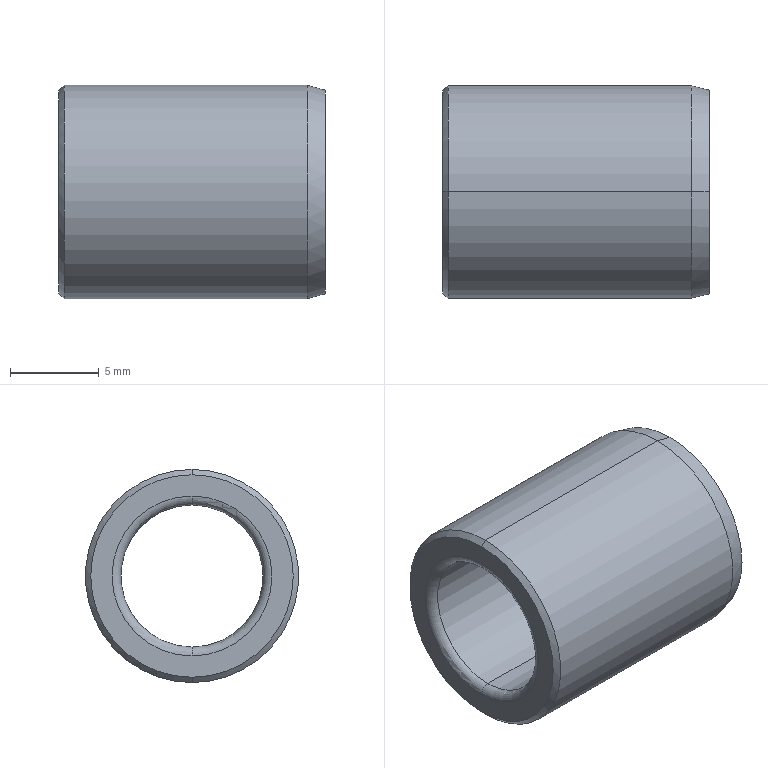Part | NX | features BREP 1 | 1 solid | 14 faces | box 15 x 12 x 12 mm | volume 933.062 mm3 | cylinder 4 | cone 4 | torus 4 | plane 2 | commonest cylinder face diameters 8 x2 12 x2
STEP:
#1=CARTESIAN_POINT('',(14.,0.,6.));
#2=VERTEX_POINT('',#1);
#3=CARTESIAN_POINT('',(14.,0.,-6.));
#4=VERTEX_POINT('',#3);
#5=CARTESIAN_POINT('',(14.,0.,0.));
#6=DIRECTION('',(-1.,0.,0.));
#7=DIRECTION('',(0.,0.,1.));
#8=AXIS2_PLACEMENT_3D('',#5,#6,#7);
#9=CIRCLE('',#8,6.);
#10=EDGE_CURVE('',#2,#4,#9,.T.);
#11=ORIENTED_EDGE('',*,*,#10,.T.);
#12=CARTESIAN_POINT('',(0.3,0.,-6.));
#13=VERTEX_POINT('',#12);
#14=CARTESIAN_POINT('',(15.,0.,-6.));
#15=DIRECTION('',(-1.,0.,0.));
#16=VECTOR('',#15,1000.);
#17=LINE('',#14,#16);
#18=EDGE_CURVE('',#13,#4,#17,.F.);
#19=ORIENTED_EDGE('',*,*,#18,.F.);
#20=CARTESIAN_POINT('',(0.3,0.,6.));
#21=VERTEX_POINT('',#20);
#22=CARTESIAN_POINT('',(0.3,0.,0.));
#23=DIRECTION('',(-1.,0.,0.));
#24=DIRECTION('',(0.,0.,1.));
#25=AXIS2_PLACEMENT_3D('',#22,#23,#24);
#26=CIRCLE('',#25,6.);
#27=EDGE_CURVE('',#21,#13,#26,.T.);
#28=ORIENTED_EDGE('',*,*,#27,.F.);
#29=CARTESIAN_POINT('',(15.,0.,6.));
#30=DIRECTION('',(-1.,0.,0.));
#31=VECTOR('',#30,1000.);
#32=LINE('',#29,#31);
#33=EDGE_CURVE('',#21,#2,#32,.F.);
#34=ORIENTED_EDGE('',*,*,#33,.T.);
#35=EDGE_LOOP('',(#11,#19,#28,#34));
#36=FACE_BOUND('',#35,.T.);
#37=CARTESIAN_POINT('',(15.,0.,0.));
#38=DIRECTION('',(-1.,0.,0.));
#39=DIRECTION('',(0.,0.,1.));
#40=AXIS2_PLACEMENT_3D('',#37,#38,#39);
#41=CYLINDRICAL_SURFACE('',#40,6.);
#42=ADVANCED_FACE('',(#36),#41,.T.);
#43=CARTESIAN_POINT('',(15.,0.,5.732));
#44=VERTEX_POINT('',#43);
#45=CARTESIAN_POINT('',(15.,0.,-5.732));
#46=VERTEX_POINT('',#45);
#47=CARTESIAN_POINT('',(15.,0.,0.));
#48=DIRECTION('',(-1.,0.,0.));
#49=DIRECTION('',(0.,0.,1.));
#50=AXIS2_PLACEMENT_3D('',#47,#48,#49);
#51=CIRCLE('',#50,5.732);
#52=EDGE_CURVE('',#44,#46,#51,.T.);
#53=ORIENTED_EDGE('',*,*,#52,.T.);
#54=CARTESIAN_POINT('',(15.,0.,-5.732));
#55=DIRECTION('',(-0.9659,0.,-0.2588));
#56=VECTOR('',#55,1000.);
#57=LINE('',#54,#56);
#58=EDGE_CURVE('',#4,#46,#57,.F.);
#59=ORIENTED_EDGE('',*,*,#58,.F.);
#60=ORIENTED_EDGE('',*,*,#10,.F.);
#61=CARTESIAN_POINT('',(15.,0.,5.732));
#62=DIRECTION('',(-0.9659,0.,0.2588));
#63=VECTOR('',#62,1000.);
#64=LINE('',#61,#63);
#65=EDGE_CURVE('',#2,#44,#64,.F.);
#66=ORIENTED_EDGE('',*,*,#65,.T.);
#67=EDGE_LOOP('',(#53,#59,#60,#66));
#68=FACE_BOUND('',#67,.T.);
#69=CARTESIAN_POINT('',(15.,0.,0.));
#70=DIRECTION('',(-1.,0.,0.));
#71=DIRECTION('',(0.,0.,1.));
#72=AXIS2_PLACEMENT_3D('',#69,#70,#71);
#73=CONICAL_SURFACE('',#72,5.732,0.2618);
#74=ADVANCED_FACE('',(#68),#73,.T.);
#75=CARTESIAN_POINT('',(14.5,0.,4.));
#76=VERTEX_POINT('',#75);
#77=CARTESIAN_POINT('',(14.5,0.,-4.));
#78=VERTEX_POINT('',#77);
#79=CARTESIAN_POINT('',(14.5,0.,0.));
#80=DIRECTION('',(-1.,0.,0.));
#81=DIRECTION('',(0.,0.,1.));
#82=AXIS2_PLACEMENT_3D('',#79,#80,#81);
#83=CIRCLE('',#82,4.);
#84=EDGE_CURVE('',#76,#78,#83,.T.);
#85=ORIENTED_EDGE('',*,*,#84,.T.);
#86=CARTESIAN_POINT('',(15.,0.,-4.5));
#87=VERTEX_POINT('',#86);
#88=CARTESIAN_POINT('',(14.5,0.,-4.5));
#89=DIRECTION('',(0.,1.,0.));
#90=DIRECTION('',(0.,0.,1.));
#91=AXIS2_PLACEMENT_3D('',#88,#89,#90);
#92=CIRCLE('',#91,0.5);
#93=EDGE_CURVE('',#87,#78,#92,.F.);
#94=ORIENTED_EDGE('',*,*,#93,.F.);
#95=CARTESIAN_POINT('',(15.,0.,4.5));
#96=VERTEX_POINT('',#95);
#97=CARTESIAN_POINT('',(15.,0.,0.));
#98=DIRECTION('',(-1.,0.,0.));
#99=DIRECTION('',(0.,0.,1.));
#100=AXIS2_PLACEMENT_3D('',#97,#98,#99);
#101=CIRCLE('',#100,4.5);
#102=EDGE_CURVE('',#96,#87,#101,.T.);
#103=ORIENTED_EDGE('',*,*,#102,.F.);
#104=CARTESIAN_POINT('',(14.5,0.,4.5));
#105=DIRECTION('',(0.,-1.,0.));
#106=DIRECTION('',(0.,0.,-1.));
#107=AXIS2_PLACEMENT_3D('',#104,#105,#106);
#108=CIRCLE('',#107,0.5);
#109=EDGE_CURVE('',#96,#76,#108,.F.);
#110=ORIENTED_EDGE('',*,*,#109,.T.);
#111=EDGE_LOOP('',(#85,#94,#103,#110));
#112=FACE_BOUND('',#111,.T.);
#113=CARTESIAN_POINT('',(14.5,0.,0.));
#114=DIRECTION('',(-1.,0.,0.));
#115=DIRECTION('',(0.,0.,1.));
#116=AXIS2_PLACEMENT_3D('',#113,#114,#115);
#117=TOROIDAL_SURFACE('',#116,4.5,0.5);
#118=ADVANCED_FACE('',(#112),#117,.T.);
#119=CARTESIAN_POINT('',(14.5,0.,0.));
#120=DIRECTION('',(-1.,0.,0.));
#121=DIRECTION('',(0.,0.,1.));
#122=AXIS2_PLACEMENT_3D('',#119,#120,#121);
#123=CIRCLE('',#122,4.);
#124=EDGE_CURVE('',#78,#76,#123,.T.);
#125=ORIENTED_EDGE('',*,*,#124,.F.);
#126=CARTESIAN_POINT('',(0.5,0.,-4.));
#127=VERTEX_POINT('',#126);
#128=CARTESIAN_POINT('',(15.,0.,-4.));
#129=DIRECTION('',(-1.,0.,0.));
#130=VECTOR('',#129,1000.);
#131=LINE('',#128,#130);
#132=EDGE_CURVE('',#127,#78,#131,.F.);
#133=ORIENTED_EDGE('',*,*,#132,.F.);
#134=CARTESIAN_POINT('',(0.5,0.,4.));
#135=VERTEX_POINT('',#134);
#136=CARTESIAN_POINT('',(0.5,0.,0.));
#137=DIRECTION('',(-1.,0.,0.));
#138=DIRECTION('',(0.,0.,1.));
#139=AXIS2_PLACEMENT_3D('',#136,#137,#138);
#140=CIRCLE('',#139,4.);
#141=EDGE_CURVE('',#127,#135,#140,.T.);
#142=ORIENTED_EDGE('',*,*,#141,.T.);
#143=CARTESIAN_POINT('',(15.,0.,4.));
#144=DIRECTION('',(-1.,0.,0.));
#145=VECTOR('',#144,1000.);
#146=LINE('',#143,#145);
#147=EDGE_CURVE('',#135,#76,#146,.F.);
#148=ORIENTED_EDGE('',*,*,#147,.T.);
#149=EDGE_LOOP('',(#125,#133,#142,#148));
#150=FACE_BOUND('',#149,.T.);
#151=CARTESIAN_POINT('',(15.,0.,0.));
#152=DIRECTION('',(-1.,0.,0.));
#153=DIRECTION('',(0.,0.,1.));
#154=AXIS2_PLACEMENT_3D('',#151,#152,#153);
#155=CYLINDRICAL_SURFACE('',#154,4.);
#156=ADVANCED_FACE('',(#150),#155,.F.);
#157=CARTESIAN_POINT('',(0.,0.,4.5));
#158=VERTEX_POINT('',#157);
#159=CARTESIAN_POINT('',(0.,0.,-4.5));
#160=VERTEX_POINT('',#159);
#161=CARTESIAN_POINT('',(0.,0.,0.));
#162=DIRECTION('',(-1.,0.,0.));
#163=DIRECTION('',(0.,0.,1.));
#164=AXIS2_PLACEMENT_3D('',#161,#162,#163);
#165=CIRCLE('',#164,4.5);
#166=EDGE_CURVE('',#158,#160,#165,.T.);
#167=ORIENTED_EDGE('',*,*,#166,.T.);
#168=CARTESIAN_POINT('',(0.5,0.,-4.5));
#169=DIRECTION('',(0.,1.,0.));
#170=DIRECTION('',(0.,0.,1.));
#171=AXIS2_PLACEMENT_3D('',#168,#169,#170);
#172=CIRCLE('',#171,0.5);
#173=EDGE_CURVE('',#127,#160,#172,.F.);
#174=ORIENTED_EDGE('',*,*,#173,.F.);
#175=CARTESIAN_POINT('',(0.5,0.,0.));
#176=DIRECTION('',(-1.,0.,0.));
#177=DIRECTION('',(0.,0.,1.));
#178=AXIS2_PLACEMENT_3D('',#175,#176,#177);
#179=CIRCLE('',#178,4.);
#180=EDGE_CURVE('',#135,#127,#179,.T.);
#181=ORIENTED_EDGE('',*,*,#180,.F.);
#182=CARTESIAN_POINT('',(0.5,0.,4.5));
#183=DIRECTION('',(0.,-1.,0.));
#184=DIRECTION('',(0.,0.,-1.));
#185=AXIS2_PLACEMENT_3D('',#182,#183,#184);
#186=CIRCLE('',#185,0.5);
#187=EDGE_CURVE('',#135,#158,#186,.F.);
#188=ORIENTED_EDGE('',*,*,#187,.T.);
#189=EDGE_LOOP('',(#167,#174,#181,#188));
#190=FACE_BOUND('',#189,.T.);
#191=CARTESIAN_POINT('',(0.5,0.,0.));
#192=DIRECTION('',(-1.,0.,0.));
#193=DIRECTION('',(0.,0.,1.));
#194=AXIS2_PLACEMENT_3D('',#191,#192,#193);
#195=TOROIDAL_SURFACE('',#194,4.5,0.5);
#196=ADVANCED_FACE('',(#190),#195,.T.);
#197=CARTESIAN_POINT('',(0.,0.,5.7));
#198=VERTEX_POINT('',#197);
#199=CARTESIAN_POINT('',(0.,0.,-5.7));
#200=VERTEX_POINT('',#199);
#201=CARTESIAN_POINT('',(0.,0.,0.));
#202=DIRECTION('',(-1.,0.,0.));
#203=DIRECTION('',(0.,0.,1.));
#204=AXIS2_PLACEMENT_3D('',#201,#202,#203);
#205=CIRCLE('',#204,5.7);
#206=EDGE_CURVE('',#198,#200,#205,.T.);
#207=ORIENTED_EDGE('',*,*,#206,.F.);
#208=CARTESIAN_POINT('',(0.3,0.,6.));
#209=DIRECTION('',(0.7071,0.,0.7071));
#210=VECTOR('',#209,1000.);
#211=LINE('',#208,#210);
#212=EDGE_CURVE('',#198,#21,#211,.T.);
#213=ORIENTED_EDGE('',*,*,#212,.T.);
#214=ORIENTED_EDGE('',*,*,#27,.T.);
#215=CARTESIAN_POINT('',(0.3,0.,-6.));
#216=DIRECTION('',(0.7071,0.,-0.7071));
#217=VECTOR('',#216,1000.);
#218=LINE('',#215,#217);
#219=EDGE_CURVE('',#200,#13,#218,.T.);
#220=ORIENTED_EDGE('',*,*,#219,.F.);
#221=EDGE_LOOP('',(#207,#213,#214,#220));
#222=FACE_BOUND('',#221,.T.);
#223=CARTESIAN_POINT('',(0.3,0.,0.));
#224=DIRECTION('',(1.,0.,0.));
#225=DIRECTION('',(0.,0.,-1.));
#226=AXIS2_PLACEMENT_3D('',#223,#224,#225);
#227=CONICAL_SURFACE('',#226,6.,0.7854);
#228=ADVANCED_FACE('',(#222),#227,.T.);
#229=ORIENTED_EDGE('',*,*,#212,.F.);
#230=CARTESIAN_POINT('',(0.,0.,0.));
#231=DIRECTION('',(-1.,0.,0.));
#232=DIRECTION('',(0.,0.,1.));
#233=AXIS2_PLACEMENT_3D('',#230,#231,#232);
#234=CIRCLE('',#233,5.7);
#235=EDGE_CURVE('',#200,#198,#234,.T.);
#236=ORIENTED_EDGE('',*,*,#235,.F.);
#237=ORIENTED_EDGE('',*,*,#219,.T.);
#238=CARTESIAN_POINT('',(0.3,0.,0.));
#239=DIRECTION('',(-1.,0.,0.));
#240=DIRECTION('',(0.,0.,1.));
#241=AXIS2_PLACEMENT_3D('',#238,#239,#240);
#242=CIRCLE('',#241,6.);
#243=EDGE_CURVE('',#13,#21,#242,.T.);
#244=ORIENTED_EDGE('',*,*,#243,.T.);
#245=EDGE_LOOP('',(#229,#236,#237,#244));
#246=FACE_BOUND('',#245,.T.);
#247=CARTESIAN_POINT('',(0.3,0.,0.));
#248=DIRECTION('',(1.,0.,0.));
#249=DIRECTION('',(0.,0.,-1.));
#250=AXIS2_PLACEMENT_3D('',#247,#248,#249);
#251=CONICAL_SURFACE('',#250,6.,0.7854);
#252=ADVANCED_FACE('',(#246),#251,.T.);
#253=ORIENTED_EDGE('',*,*,#235,.T.);
#254=ORIENTED_EDGE('',*,*,#206,.T.);
#255=EDGE_LOOP('',(#253,#254));
#256=FACE_BOUND('',#255,.T.);
#257=ORIENTED_EDGE('',*,*,#166,.F.);
#258=CARTESIAN_POINT('',(0.,0.,0.));
#259=DIRECTION('',(-1.,0.,0.));
#260=DIRECTION('',(0.,0.,1.));
#261=AXIS2_PLACEMENT_3D('',#258,#259,#260);
#262=CIRCLE('',#261,4.5);
#263=EDGE_CURVE('',#160,#158,#262,.T.);
#264=ORIENTED_EDGE('',*,*,#263,.F.);
#265=EDGE_LOOP('',(#257,#264));
#266=FACE_BOUND('',#265,.T.);
#267=CARTESIAN_POINT('',(0.,5.7,0.));
#268=DIRECTION('',(1.,0.,0.));
#269=DIRECTION('',(0.,1.,0.));
#270=AXIS2_PLACEMENT_3D('',#267,#268,#269);
#271=PLANE('',#270);
#272=ADVANCED_FACE('',(#256,#266),#271,.F.);
#273=ORIENTED_EDGE('',*,*,#173,.T.);
#274=ORIENTED_EDGE('',*,*,#263,.T.);
#275=ORIENTED_EDGE('',*,*,#187,.F.);
#276=ORIENTED_EDGE('',*,*,#141,.F.);
#277=EDGE_LOOP('',(#273,#274,#275,#276));
#278=FACE_BOUND('',#277,.T.);
#279=CARTESIAN_POINT('',(0.5,0.,0.));
#280=DIRECTION('',(-1.,0.,0.));
#281=DIRECTION('',(0.,0.,1.));
#282=AXIS2_PLACEMENT_3D('',#279,#280,#281);
#283=TOROIDAL_SURFACE('',#282,4.5,0.5);
#284=ADVANCED_FACE('',(#278),#283,.T.);
#285=ORIENTED_EDGE('',*,*,#132,.T.);
#286=ORIENTED_EDGE('',*,*,#84,.F.);
#287=ORIENTED_EDGE('',*,*,#147,.F.);
#288=ORIENTED_EDGE('',*,*,#180,.T.);
#289=EDGE_LOOP('',(#285,#286,#287,#288));
#290=FACE_BOUND('',#289,.T.);
#291=CARTESIAN_POINT('',(15.,0.,0.));
#292=DIRECTION('',(-1.,0.,0.));
#293=DIRECTION('',(0.,0.,1.));
#294=AXIS2_PLACEMENT_3D('',#291,#292,#293);
#295=CYLINDRICAL_SURFACE('',#294,4.);
#296=ADVANCED_FACE('',(#290),#295,.F.);
#297=ORIENTED_EDGE('',*,*,#93,.T.);
#298=ORIENTED_EDGE('',*,*,#124,.T.);
#299=ORIENTED_EDGE('',*,*,#109,.F.);
#300=CARTESIAN_POINT('',(15.,0.,0.));
#301=DIRECTION('',(-1.,0.,0.));
#302=DIRECTION('',(0.,0.,1.));
#303=AXIS2_PLACEMENT_3D('',#300,#301,#302);
#304=CIRCLE('',#303,4.5);
#305=EDGE_CURVE('',#87,#96,#304,.T.);
#306=ORIENTED_EDGE('',*,*,#305,.F.);
#307=EDGE_LOOP('',(#297,#298,#299,#306));
#308=FACE_BOUND('',#307,.T.);
#309=CARTESIAN_POINT('',(14.5,0.,0.));
#310=DIRECTION('',(-1.,0.,0.));
#311=DIRECTION('',(0.,0.,1.));
#312=AXIS2_PLACEMENT_3D('',#309,#310,#311);
#313=TOROIDAL_SURFACE('',#312,4.5,0.5);
#314=ADVANCED_FACE('',(#308),#313,.T.);
#315=ORIENTED_EDGE('',*,*,#52,.F.);
#316=CARTESIAN_POINT('',(15.,0.,0.));
#317=DIRECTION('',(-1.,0.,0.));
#318=DIRECTION('',(0.,0.,1.));
#319=AXIS2_PLACEMENT_3D('',#316,#317,#318);
#320=CIRCLE('',#319,5.732);
#321=EDGE_CURVE('',#46,#44,#320,.T.);
#322=ORIENTED_EDGE('',*,*,#321,.F.);
#323=EDGE_LOOP('',(#315,#322));
#324=FACE_BOUND('',#323,.T.);
#325=ORIENTED_EDGE('',*,*,#102,.T.);
#326=ORIENTED_EDGE('',*,*,#305,.T.);
#327=EDGE_LOOP('',(#325,#326));
#328=FACE_BOUND('',#327,.T.);
#329=CARTESIAN_POINT('',(15.,4.5,0.));
#330=DIRECTION('',(-1.,0.,0.));
#331=DIRECTION('',(0.,0.,1.));
#332=AXIS2_PLACEMENT_3D('',#329,#330,#331);
#333=PLANE('',#332);
#334=ADVANCED_FACE('',(#324,#328),#333,.F.);
#335=ORIENTED_EDGE('',*,*,#58,.T.);
#336=ORIENTED_EDGE('',*,*,#321,.T.);
#337=ORIENTED_EDGE('',*,*,#65,.F.);
#338=CARTESIAN_POINT('',(14.,0.,0.));
#339=DIRECTION('',(-1.,0.,0.));
#340=DIRECTION('',(0.,0.,1.));
#341=AXIS2_PLACEMENT_3D('',#338,#339,#340);
#342=CIRCLE('',#341,6.);
#343=EDGE_CURVE('',#4,#2,#342,.T.);
#344=ORIENTED_EDGE('',*,*,#343,.F.);
#345=EDGE_LOOP('',(#335,#336,#337,#344));
#346=FACE_BOUND('',#345,.T.);
#347=CARTESIAN_POINT('',(15.,0.,0.));
#348=DIRECTION('',(-1.,0.,0.));
#349=DIRECTION('',(0.,0.,1.));
#350=AXIS2_PLACEMENT_3D('',#347,#348,#349);
#351=CONICAL_SURFACE('',#350,5.732,0.2618);
#352=ADVANCED_FACE('',(#346),#351,.T.);
#353=ORIENTED_EDGE('',*,*,#18,.T.);
#354=ORIENTED_EDGE('',*,*,#343,.T.);
#355=ORIENTED_EDGE('',*,*,#33,.F.);
#356=ORIENTED_EDGE('',*,*,#243,.F.);
#357=EDGE_LOOP('',(#353,#354,#355,#356));
#358=FACE_BOUND('',#357,.T.);
#359=CARTESIAN_POINT('',(15.,0.,0.));
#360=DIRECTION('',(-1.,0.,0.));
#361=DIRECTION('',(0.,0.,1.));
#362=AXIS2_PLACEMENT_3D('',#359,#360,#361);
#363=CYLINDRICAL_SURFACE('',#362,6.);
#364=ADVANCED_FACE('',(#358),#363,.T.);
#365=CLOSED_SHELL('',(#42,#74,#118,#156,#196,#228,#252,#272,#284,#296,#314,#334,#352,#364));
#366=MANIFOLD_SOLID_BREP('',#365);
#367=(LENGTH_UNIT()NAMED_UNIT(*)SI_UNIT(.MILLI.,.METRE.));
#368=UNCERTAINTY_MEASURE_WITH_UNIT(LENGTH_MEASURE(0.00001),#367,'','');
#369=(NAMED_UNIT(*)PLANE_ANGLE_UNIT()SI_UNIT($,.RADIAN.));
#370=(NAMED_UNIT(*)SI_UNIT($,.STERADIAN.)SOLID_ANGLE_UNIT());
#371=(GEOMETRIC_REPRESENTATION_CONTEXT(3)GLOBAL_UNCERTAINTY_ASSIGNED_CONTEXT((#368))GLOBAL_UNIT_ASSIGNED_CONTEXT((#367,#369,#370))REPRESENTATION_CONTEXT('',''));
#372=ADVANCED_BREP_SHAPE_REPRESENTATION('',(#366),#371);